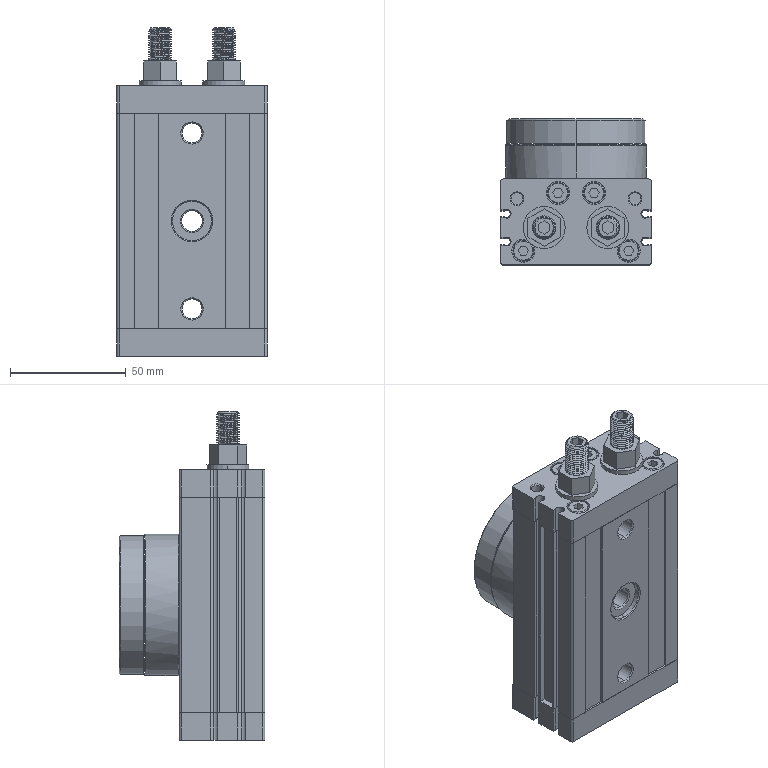Part | SolidWorks | features ICE 19, MirrorPattern 7, Chamfer 6, Revolution 4, Fillet 3, MirrorSolid 3, CirPattern 2, DeleteBody 2, Helix 2, RevCut 2, SweepCut 2, Extrusion 1, SketchPattern 1 | 6 solids | 560 faces | box 65 x 63 x 142 mm | volume 327794 mm3 | plane 272 | cylinder 199 | cone 49 | torus 32 | spline 8 | commonest cylinder face diameters 10 x56 6 x24 9.007 x16 10.007 x16 2 x12 3.865 x12